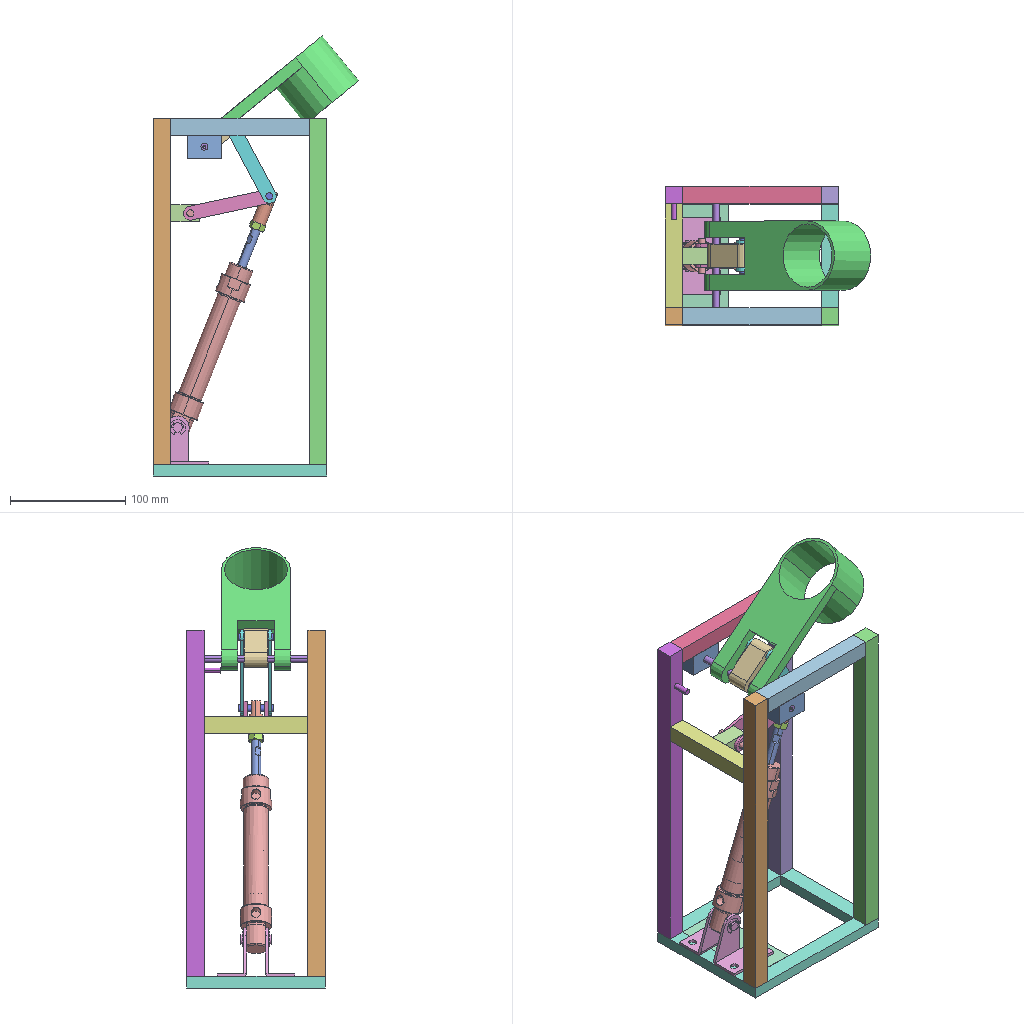Assembly | SolidWorks | 16 different items | 20 placed | box 178 x 120 x 381 mm
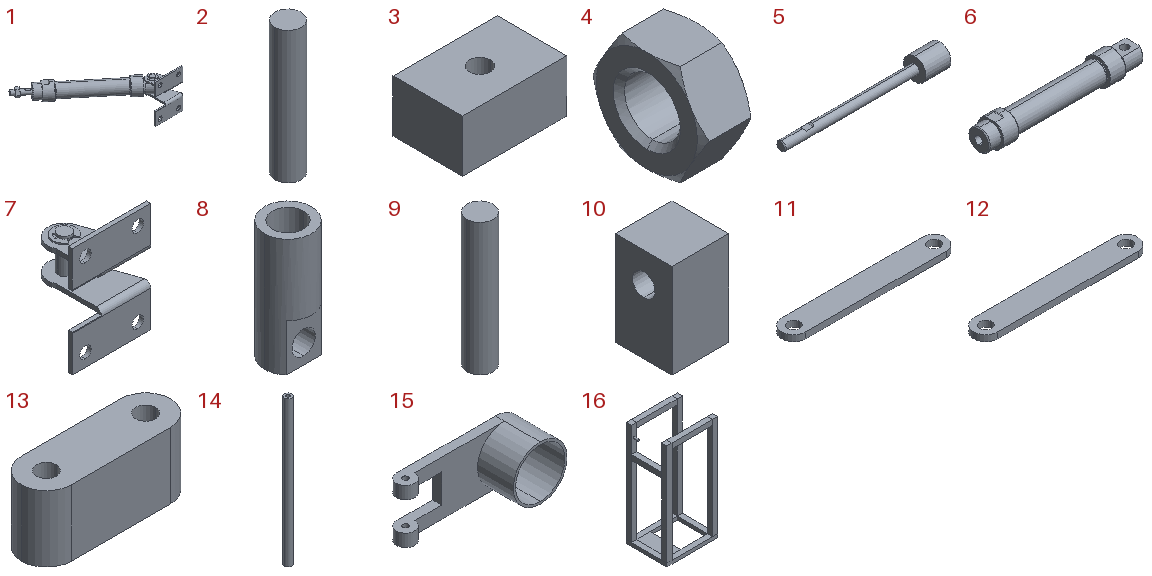Parts list (item | name | quantity | parent item | size | volume | features):
1 | (subassembly) | x1 | - | 160.322 x 147.922 x 67 mm | 60763 mm3 | features CompositeCurve 1
2 | - | x1 | - | 6 x 6 x 30 mm | 848.23 mm3 | features Extrusion 1
3 | - | x2 | - | 30 x 20 x 15 mm | 8576 mm3 | features Extrusion 1, ICE 1
4 | - | x1 | in 1 | 6 x 13.856 x 12 mm | 526.038 mm3 | features BaseBody 1
5 | - | x1 | in 1 | 139 x 19.5 x 19.5 mm | 12392 mm3 | features BaseBody 1
6 | - | x1 | in 1 | 159 x 27 x 27 mm | 36878 mm3 | features BaseBody 1
7 | - | x1 | in 1 | 48 x 42 x 67 mm | 10967 mm3 | features BaseBody 1
8 | - | x1 | - | 12 x 12 x 30 mm | 2367 mm3 | features ICE 3, Extrusion 1, MirrorPattern 1
9 | - | x2 | - | 6 x 6 x 30 mm | 848.23 mm3 | features Extrusion 1
10 | - | x1 | - | 15 x 15 x 25 mm | 5201 mm3 | features Cut 1, Extrusion 1
11 | - | x2 | - | 82 x 12 x 3 mm | 2690 mm3 | features Extrusion 1
12 | - | x2 | - | 82 x 12 x 3 mm | 2690 mm3 | features Extrusion 1
13 | - | x1 | - | 45 x 15 x 20 mm | 11403 mm3 | features Extrusion 1
14 | - | x1 | - | 6 x 6 x 120 mm | 3307 mm3 | features HoleWzd 2, Extrusion 1
15 | - | x1 | - | 150 x 50 x 60 mm | 67449 mm3 | features ICE 4, Extrusion 1
16 | - | x1 | - | 150 x 120 x 310 mm | 427325 mm3 | features ICE 6, Extrusion 1
Mates (type | each side: item.copy, entity, surface, feature):
In the top assembly
Coincident | 16.1 face plane Boss-Extrude1 | 7.1 face plane Input1 | 2 times
Width | 16.1 face plane Boss-Extrude2 | 16.1 face plane Boss-Extrude2 | 7.1 face plane Input1 | 7.1 face plane Input1
Coincident | 16.1 face plane Boss-Extrude7 | 3.1 face plane Boss-Extrude1 | 2 times
Concentric | 3.1 face cylinder Cut-Extrude1 | 3.2 face cylinder Cut-Extrude1
Coincident | 16.1 face plane Boss-Extrude7 | 3.2 face plane Boss-Extrude1
Coincident | 3.1 face plane Boss-Extrude1 | 3.2 face plane Boss-Extrude1
Concentric | 3.2 face cylinder Cut-Extrude1 | 14.1 face cylinder Boss-Extrude1
Width | 14.1 face plane Boss-Extrude1 | 14.1 face plane Boss-Extrude1 | 16.1 face plane Boss-Extrude7 | 16.1 face plane Boss-Extrude7
Concentric | 5.1 face cylinder Input1 | 8.1 face cylinder Cut-Extrude3
Coincident | 4.1 face plane Input1 | 8.1 face plane Boss-Extrude1
Concentric | 8.1 face cylinder Cut-Extrude2 | 9.1 face cylinder Boss-Extrude1
Parallel | 6.1 face plane Input1 | 8.1 face plane Mirror1
Width | 9.1 face plane Boss-Extrude1 | 9.1 face plane Boss-Extrude1 | 8.1 face plane Cut-Extrude1 | 8.1 face plane Mirror1
Coincident | 16.1 face plane Boss-Extrude8 | 10.1 face plane Boss-Extrude1 | 2 times
Width | 16.1 face plane Boss-Extrude2 | 16.1 face plane Boss-Extrude2 | 10.1 face plane Boss-Extrude1 | 10.1 face plane Boss-Extrude1
Concentric | 10.1 face cylinder Cut-Extrude1 | 2.1 face cylinder Boss-Extrude1
Width | 2.1 face plane Boss-Extrude1 | 2.1 face plane Boss-Extrude1 | 10.1 face plane Boss-Extrude1 | 10.1 face plane Boss-Extrude1
Concentric | 2.1 face cylinder Boss-Extrude1 | 11.1 face cylinder Boss-Extrude1
Coincident | 10.1 face plane Boss-Extrude1 | 11.1 face plane Boss-Extrude1
Concentric | 9.1 face cylinder Boss-Extrude1 | 11.1 face cylinder Boss-Extrude1
Concentric | 2.1 face cylinder Boss-Extrude1 | 11.2 face cylinder Boss-Extrude1
Concentric | 9.1 face cylinder Boss-Extrude1 | 11.2 face cylinder Boss-Extrude1
Coincident | 10.1 face plane Boss-Extrude1 | 11.2 face plane Boss-Extrude1
Concentric | 9.1 face cylinder Boss-Extrude1 | 12.1 face cylinder Boss-Extrude1
Coincident | 11.2 face plane Boss-Extrude1 | 12.1 face plane Boss-Extrude1
Concentric | 9.1 face cylinder Boss-Extrude1 | 12.2 face cylinder Boss-Extrude1
Coincident | 11.1 face plane Boss-Extrude1 | 12.2 face plane Boss-Extrude1
Concentric | 12.1 face cylinder Boss-Extrude1 | 12.2 face cylinder Boss-Extrude1
Concentric | 14.1 face cylinder Boss-Extrude1 | 13.1 face cylinder Boss-Extrude1
Width | 12.1 face plane Boss-Extrude1 | 12.2 face plane Boss-Extrude1 | 13.1 face plane Boss-Extrude1 | 13.1 face plane Boss-Extrude1
Concentric | 12.1 face cylinder Boss-Extrude1 | 9.2 face cylinder Boss-Extrude1
Width | 9.2 face plane Boss-Extrude1 | 9.2 face plane Boss-Extrude1 | 12.2 face plane Boss-Extrude1 | 12.1 face plane Boss-Extrude1
Concentric | 13.1 face cylinder Boss-Extrude1 | 9.2 face cylinder Boss-Extrude1
Width | 16.1 face plane Boss-Extrude7 | 16.1 face plane Boss-Extrude7 | 15.1 face plane Boss-Extrude1 | 15.1 face plane Boss-Extrude1
Concentric | 13.1 face cylinder Boss-Extrude1 | 15.1 face cylinder Boss-Extrude1
Parallel | 13.1 face plane Boss-Extrude1 | 15.1 face plane Boss-Extrude2
DistanceDim | 16.1 face plane Boss-Extrude2 | 3.1 face plane Boss-Extrude1
In subassembly 1
Concentric | 5.2 face cylinder Input1 | 4.2 edge
DistanceDim | 4.2 face plane Input1 | 5.2 face plane Input1
Concentric | 6.2 face cylinder Input1 | 7.2 face cylinder Input1
Width | 7.2 face plane Input1 | 7.2 face plane Input1 | 6.2 face plane Input1 | 6.2 face plane Input1
Concentric | 6.2 face cylinder Input1 | 5.2 face cylinder Input1 | 2 times
LimitDistanceDim | 5.2 face plane Input1 | 6.2 face plane Input1